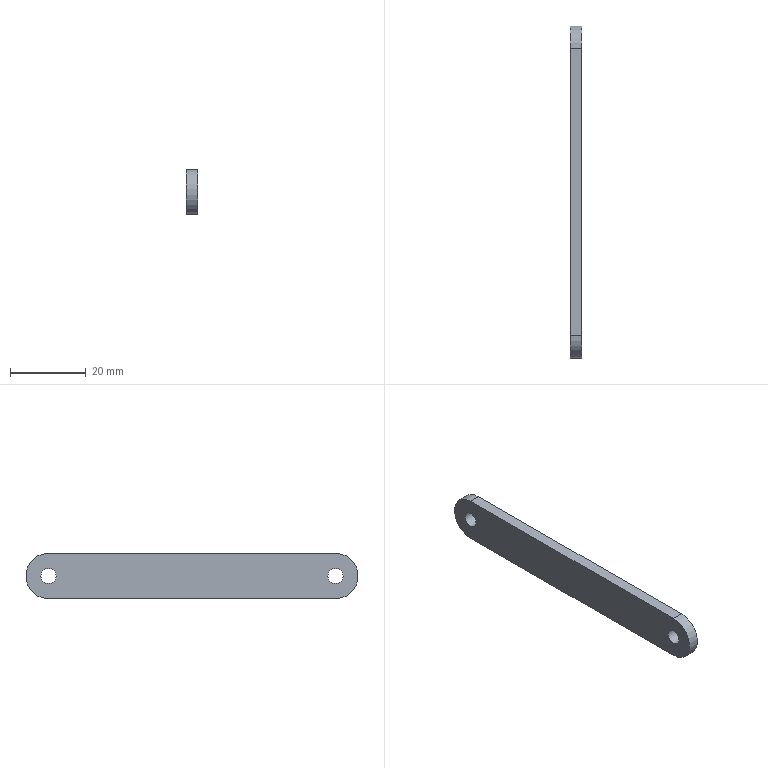Part | STEP file | 1-46.10 | 1 solid | 8 faces | box 3 x 88 x 12 mm | volume 3000 mm3 | plane 4 | cylinder 4 | commonest cylinder face diameters 4 x2 12 x2
STEP:
#1=CARTESIAN_POINT('',(0.,0.,0.));
#2=DIRECTION('',(0.,0.,1.));
#3=DIRECTION('',(1.,0.,0.));
#4=AXIS2_PLACEMENT_3D('',#1,#2,#3);
#5=CARTESIAN_POINT('',(0.,-38.,6.));
#6=VERTEX_POINT('',#5);
#7=CARTESIAN_POINT('',(0.,-38.,-6.));
#8=VERTEX_POINT('',#7);
#9=CARTESIAN_POINT('',(0.,-38.,0.));
#10=DIRECTION('',(1.,0.,0.));
#11=DIRECTION('',(0.,0.,1.));
#12=AXIS2_PLACEMENT_3D('',#9,#10,#11);
#13=CIRCLE('',#12,6.);
#14=CARTESIAN_POINT('',(0.,0.,38.));
#15=DIRECTION('',(1.,0.,0.));
#16=DIRECTION('',(0.,1.,0.));
#17=AXIS2_PLACEMENT_3D('',#14,#15,#16);
#18=PLANE('',#17);
#19=CARTESIAN_POINT('',(-38.,-38.));
#20=DIRECTION('',(0.,1.));
#21=AXIS2_PLACEMENT_2D('',#19,#20);
#22=CIRCLE('',#21,6.);
#23=(GEOMETRIC_REPRESENTATION_CONTEXT(2)PARAMETRIC_REPRESENTATION_CONTEXT()REPRESENTATION_CONTEXT('',''));
#24=DEFINITIONAL_REPRESENTATION('',(#22),#23);
#25=PCURVE('',#18,#24);
#26=CARTESIAN_POINT('',(0.,-38.,0.));
#27=DIRECTION('',(1.,0.,0.));
#28=DIRECTION('',(0.,0.,1.));
#29=AXIS2_PLACEMENT_3D('',#26,#27,#28);
#30=CYLINDRICAL_SURFACE('',#29,6.);
#31=CARTESIAN_POINT('',(0.,0.));
#32=DIRECTION('',(1.,0.));
#33=VECTOR('',#32,1.);
#34=LINE('',#31,#33);
#35=(GEOMETRIC_REPRESENTATION_CONTEXT(2)PARAMETRIC_REPRESENTATION_CONTEXT()REPRESENTATION_CONTEXT('',''));
#36=DEFINITIONAL_REPRESENTATION('',(#34),#35);
#37=PCURVE('',#30,#36);
#38=SURFACE_CURVE('',#13,(#25,#37),.PCURVE_S1.);
#39=EDGE_CURVE('',#6,#8,#38,.T.);
#40=ORIENTED_EDGE('',*,*,#39,.T.);
#41=CARTESIAN_POINT('',(0.,38.,-6.));
#42=VERTEX_POINT('',#41);
#43=CARTESIAN_POINT('',(0.,-38.,-6.));
#44=DIRECTION('',(0.,1.,0.));
#45=VECTOR('',#44,1.);
#46=LINE('',#43,#45);
#47=CARTESIAN_POINT('',(-38.,-44.));
#48=DIRECTION('',(1.,0.));
#49=VECTOR('',#48,1.);
#50=LINE('',#47,#49);
#51=(GEOMETRIC_REPRESENTATION_CONTEXT(2)PARAMETRIC_REPRESENTATION_CONTEXT()REPRESENTATION_CONTEXT('',''));
#52=DEFINITIONAL_REPRESENTATION('',(#50),#51);
#53=PCURVE('',#18,#52);
#54=CARTESIAN_POINT('',(1.5,0.,-6.));
#55=DIRECTION('',(0.,0.,-1.));
#56=DIRECTION('',(0.,1.,0.));
#57=AXIS2_PLACEMENT_3D('',#54,#55,#56);
#58=PLANE('',#57);
#59=CARTESIAN_POINT('',(-38.,-1.5));
#60=DIRECTION('',(1.,0.));
#61=VECTOR('',#60,1.);
#62=LINE('',#59,#61);
#63=(GEOMETRIC_REPRESENTATION_CONTEXT(2)PARAMETRIC_REPRESENTATION_CONTEXT()REPRESENTATION_CONTEXT('',''));
#64=DEFINITIONAL_REPRESENTATION('',(#62),#63);
#65=PCURVE('',#58,#64);
#66=SURFACE_CURVE('',#46,(#53,#65),.PCURVE_S1.);
#67=EDGE_CURVE('',#8,#42,#66,.T.);
#68=ORIENTED_EDGE('',*,*,#67,.T.);
#69=CARTESIAN_POINT('',(0.,38.,6.));
#70=VERTEX_POINT('',#69);
#71=CARTESIAN_POINT('',(0.,38.,0.));
#72=DIRECTION('',(1.,0.,0.));
#73=DIRECTION('',(0.,0.,-1.));
#74=AXIS2_PLACEMENT_3D('',#71,#72,#73);
#75=CIRCLE('',#74,6.);
#76=CARTESIAN_POINT('',(38.,-38.));
#77=DIRECTION('',(0.,-1.));
#78=AXIS2_PLACEMENT_2D('',#76,#77);
#79=CIRCLE('',#78,6.);
#80=(GEOMETRIC_REPRESENTATION_CONTEXT(2)PARAMETRIC_REPRESENTATION_CONTEXT()REPRESENTATION_CONTEXT('',''));
#81=DEFINITIONAL_REPRESENTATION('',(#79),#80);
#82=PCURVE('',#18,#81);
#83=CARTESIAN_POINT('',(0.,38.,0.));
#84=DIRECTION('',(1.,0.,0.));
#85=DIRECTION('',(0.,0.,-1.));
#86=AXIS2_PLACEMENT_3D('',#83,#84,#85);
#87=CYLINDRICAL_SURFACE('',#86,6.);
#88=CARTESIAN_POINT('',(0.,0.));
#89=DIRECTION('',(1.,0.));
#90=VECTOR('',#89,1.);
#91=LINE('',#88,#90);
#92=(GEOMETRIC_REPRESENTATION_CONTEXT(2)PARAMETRIC_REPRESENTATION_CONTEXT()REPRESENTATION_CONTEXT('',''));
#93=DEFINITIONAL_REPRESENTATION('',(#91),#92);
#94=PCURVE('',#87,#93);
#95=SURFACE_CURVE('',#75,(#82,#94),.PCURVE_S1.);
#96=EDGE_CURVE('',#42,#70,#95,.T.);
#97=ORIENTED_EDGE('',*,*,#96,.T.);
#98=CARTESIAN_POINT('',(0.,38.,6.));
#99=DIRECTION('',(0.,-1.,0.));
#100=VECTOR('',#99,1.);
#101=LINE('',#98,#100);
#102=CARTESIAN_POINT('',(38.,-32.));
#103=DIRECTION('',(-1.,0.));
#104=VECTOR('',#103,1.);
#105=LINE('',#102,#104);
#106=(GEOMETRIC_REPRESENTATION_CONTEXT(2)PARAMETRIC_REPRESENTATION_CONTEXT()REPRESENTATION_CONTEXT('',''));
#107=DEFINITIONAL_REPRESENTATION('',(#105),#106);
#108=PCURVE('',#18,#107);
#109=CARTESIAN_POINT('',(1.5,0.,6.));
#110=DIRECTION('',(0.,0.,1.));
#111=DIRECTION('',(0.,-1.,0.));
#112=AXIS2_PLACEMENT_3D('',#109,#110,#111);
#113=PLANE('',#112);
#114=CARTESIAN_POINT('',(-38.,-1.5));
#115=DIRECTION('',(1.,0.));
#116=VECTOR('',#115,1.);
#117=LINE('',#114,#116);
#118=(GEOMETRIC_REPRESENTATION_CONTEXT(2)PARAMETRIC_REPRESENTATION_CONTEXT()REPRESENTATION_CONTEXT('',''));
#119=DEFINITIONAL_REPRESENTATION('',(#117),#118);
#120=PCURVE('',#113,#119);
#121=SURFACE_CURVE('',#101,(#108,#120),.PCURVE_S1.);
#122=EDGE_CURVE('',#70,#6,#121,.T.);
#123=ORIENTED_EDGE('',*,*,#122,.T.);
#124=EDGE_LOOP('',(#40,#68,#97,#123));
#125=FACE_BOUND('',#124,.F.);
#126=CARTESIAN_POINT('',(0.,-36.,0.));
#127=VERTEX_POINT('',#126);
#128=CARTESIAN_POINT('',(0.,-38.,0.));
#129=DIRECTION('',(-1.,0.,0.));
#130=DIRECTION('',(0.,1.,0.));
#131=AXIS2_PLACEMENT_3D('',#128,#129,#130);
#132=CIRCLE('',#131,2.);
#133=CARTESIAN_POINT('',(-36.,-38.));
#134=CARTESIAN_POINT('',(-36.,-41.464));
#135=CARTESIAN_POINT('',(-39.,-39.732));
#136=CARTESIAN_POINT('',(-42.,-38.));
#137=CARTESIAN_POINT('',(-39.,-36.268));
#138=CARTESIAN_POINT('',(-36.,-34.536));
#139=CARTESIAN_POINT('',(-36.,-38.));
#140=(BOUNDED_CURVE()B_SPLINE_CURVE(2,(#133,#134,#135,#136,#137,#138,#139),.UNSPECIFIED.,.T.,.F.)B_SPLINE_CURVE_WITH_KNOTS((1,2,2,2,2,1),(-2.094,0.,2.094,4.189,6.283,8.378),.UNSPECIFIED.)CURVE()GEOMETRIC_REPRESENTATION_ITEM()RATIONAL_B_SPLINE_CURVE((1.,0.5,1.,0.5,1.,0.5,1.))REPRESENTATION_ITEM(''));
#141=(GEOMETRIC_REPRESENTATION_CONTEXT(2)PARAMETRIC_REPRESENTATION_CONTEXT()REPRESENTATION_CONTEXT('',''));
#142=DEFINITIONAL_REPRESENTATION('',(#140),#141);
#143=PCURVE('',#18,#142);
#144=CARTESIAN_POINT('',(0.,-38.,0.));
#145=DIRECTION('',(1.,0.,0.));
#146=DIRECTION('',(0.,1.,0.));
#147=AXIS2_PLACEMENT_3D('',#144,#145,#146);
#148=CYLINDRICAL_SURFACE('',#147,2.);
#149=CARTESIAN_POINT('',(6.283,0.));
#150=DIRECTION('',(-1.,0.));
#151=VECTOR('',#150,1.);
#152=LINE('',#149,#151);
#153=(GEOMETRIC_REPRESENTATION_CONTEXT(2)PARAMETRIC_REPRESENTATION_CONTEXT()REPRESENTATION_CONTEXT('',''));
#154=DEFINITIONAL_REPRESENTATION('',(#152),#153);
#155=PCURVE('',#148,#154);
#156=SURFACE_CURVE('',#132,(#143,#155),.PCURVE_S1.);
#157=EDGE_CURVE('',#127,#127,#156,.T.);
#158=ORIENTED_EDGE('',*,*,#157,.T.);
#159=EDGE_LOOP('',(#158));
#160=FACE_BOUND('',#159,.F.);
#161=CARTESIAN_POINT('',(0.,40.,0.));
#162=VERTEX_POINT('',#161);
#163=CARTESIAN_POINT('',(0.,38.,0.));
#164=DIRECTION('',(-1.,0.,0.));
#165=DIRECTION('',(0.,1.,0.));
#166=AXIS2_PLACEMENT_3D('',#163,#164,#165);
#167=CIRCLE('',#166,2.);
#168=CARTESIAN_POINT('',(40.,-38.));
#169=CARTESIAN_POINT('',(40.,-41.464));
#170=CARTESIAN_POINT('',(37.,-39.732));
#171=CARTESIAN_POINT('',(34.,-38.));
#172=CARTESIAN_POINT('',(37.,-36.268));
#173=CARTESIAN_POINT('',(40.,-34.536));
#174=CARTESIAN_POINT('',(40.,-38.));
#175=(BOUNDED_CURVE()B_SPLINE_CURVE(2,(#168,#169,#170,#171,#172,#173,#174),.UNSPECIFIED.,.T.,.F.)B_SPLINE_CURVE_WITH_KNOTS((1,2,2,2,2,1),(-2.094,0.,2.094,4.189,6.283,8.378),.UNSPECIFIED.)CURVE()GEOMETRIC_REPRESENTATION_ITEM()RATIONAL_B_SPLINE_CURVE((1.,0.5,1.,0.5,1.,0.5,1.))REPRESENTATION_ITEM(''));
#176=(GEOMETRIC_REPRESENTATION_CONTEXT(2)PARAMETRIC_REPRESENTATION_CONTEXT()REPRESENTATION_CONTEXT('',''));
#177=DEFINITIONAL_REPRESENTATION('',(#175),#176);
#178=PCURVE('',#18,#177);
#179=CARTESIAN_POINT('',(0.,38.,0.));
#180=DIRECTION('',(1.,0.,0.));
#181=DIRECTION('',(0.,1.,0.));
#182=AXIS2_PLACEMENT_3D('',#179,#180,#181);
#183=CYLINDRICAL_SURFACE('',#182,2.);
#184=CARTESIAN_POINT('',(6.283,0.));
#185=DIRECTION('',(-1.,0.));
#186=VECTOR('',#185,1.);
#187=LINE('',#184,#186);
#188=(GEOMETRIC_REPRESENTATION_CONTEXT(2)PARAMETRIC_REPRESENTATION_CONTEXT()REPRESENTATION_CONTEXT('',''));
#189=DEFINITIONAL_REPRESENTATION('',(#187),#188);
#190=PCURVE('',#183,#189);
#191=SURFACE_CURVE('',#167,(#178,#190),.PCURVE_S1.);
#192=EDGE_CURVE('',#162,#162,#191,.T.);
#193=ORIENTED_EDGE('',*,*,#192,.T.);
#194=EDGE_LOOP('',(#193));
#195=FACE_BOUND('',#194,.F.);
#196=ADVANCED_FACE('',(#125,#160,#195),#18,.F.);
#197=CARTESIAN_POINT('',(3.,-38.,6.));
#198=VERTEX_POINT('',#197);
#199=CARTESIAN_POINT('',(3.,-38.,-6.));
#200=VERTEX_POINT('',#199);
#201=CARTESIAN_POINT('',(3.,-38.,0.));
#202=DIRECTION('',(1.,0.,0.));
#203=DIRECTION('',(0.,0.,1.));
#204=AXIS2_PLACEMENT_3D('',#201,#202,#203);
#205=CIRCLE('',#204,6.);
#206=CARTESIAN_POINT('',(3.,0.,38.));
#207=DIRECTION('',(1.,0.,0.));
#208=DIRECTION('',(0.,1.,0.));
#209=AXIS2_PLACEMENT_3D('',#206,#207,#208);
#210=PLANE('',#209);
#211=CARTESIAN_POINT('',(-38.,-38.));
#212=DIRECTION('',(0.,1.));
#213=AXIS2_PLACEMENT_2D('',#211,#212);
#214=CIRCLE('',#213,6.);
#215=(GEOMETRIC_REPRESENTATION_CONTEXT(2)PARAMETRIC_REPRESENTATION_CONTEXT()REPRESENTATION_CONTEXT('',''));
#216=DEFINITIONAL_REPRESENTATION('',(#214),#215);
#217=PCURVE('',#210,#216);
#218=CARTESIAN_POINT('',(0.,3.));
#219=DIRECTION('',(1.,0.));
#220=VECTOR('',#219,1.);
#221=LINE('',#218,#220);
#222=(GEOMETRIC_REPRESENTATION_CONTEXT(2)PARAMETRIC_REPRESENTATION_CONTEXT()REPRESENTATION_CONTEXT('',''));
#223=DEFINITIONAL_REPRESENTATION('',(#221),#222);
#224=PCURVE('',#30,#223);
#225=SURFACE_CURVE('',#205,(#217,#224),.PCURVE_S1.);
#226=EDGE_CURVE('',#198,#200,#225,.T.);
#227=ORIENTED_EDGE('',*,*,#226,.T.);
#228=CARTESIAN_POINT('',(3.,38.,-6.));
#229=VERTEX_POINT('',#228);
#230=CARTESIAN_POINT('',(3.,-38.,-6.));
#231=DIRECTION('',(0.,1.,0.));
#232=VECTOR('',#231,1.);
#233=LINE('',#230,#232);
#234=CARTESIAN_POINT('',(-38.,-44.));
#235=DIRECTION('',(1.,0.));
#236=VECTOR('',#235,1.);
#237=LINE('',#234,#236);
#238=(GEOMETRIC_REPRESENTATION_CONTEXT(2)PARAMETRIC_REPRESENTATION_CONTEXT()REPRESENTATION_CONTEXT('',''));
#239=DEFINITIONAL_REPRESENTATION('',(#237),#238);
#240=PCURVE('',#210,#239);
#241=CARTESIAN_POINT('',(-38.,1.5));
#242=DIRECTION('',(1.,0.));
#243=VECTOR('',#242,1.);
#244=LINE('',#241,#243);
#245=(GEOMETRIC_REPRESENTATION_CONTEXT(2)PARAMETRIC_REPRESENTATION_CONTEXT()REPRESENTATION_CONTEXT('',''));
#246=DEFINITIONAL_REPRESENTATION('',(#244),#245);
#247=PCURVE('',#58,#246);
#248=SURFACE_CURVE('',#233,(#240,#247),.PCURVE_S1.);
#249=EDGE_CURVE('',#200,#229,#248,.T.);
#250=ORIENTED_EDGE('',*,*,#249,.T.);
#251=CARTESIAN_POINT('',(3.,38.,6.));
#252=VERTEX_POINT('',#251);
#253=CARTESIAN_POINT('',(3.,38.,0.));
#254=DIRECTION('',(1.,0.,0.));
#255=DIRECTION('',(0.,0.,-1.));
#256=AXIS2_PLACEMENT_3D('',#253,#254,#255);
#257=CIRCLE('',#256,6.);
#258=CARTESIAN_POINT('',(38.,-38.));
#259=DIRECTION('',(0.,-1.));
#260=AXIS2_PLACEMENT_2D('',#258,#259);
#261=CIRCLE('',#260,6.);
#262=(GEOMETRIC_REPRESENTATION_CONTEXT(2)PARAMETRIC_REPRESENTATION_CONTEXT()REPRESENTATION_CONTEXT('',''));
#263=DEFINITIONAL_REPRESENTATION('',(#261),#262);
#264=PCURVE('',#210,#263);
#265=CARTESIAN_POINT('',(0.,3.));
#266=DIRECTION('',(1.,0.));
#267=VECTOR('',#266,1.);
#268=LINE('',#265,#267);
#269=(GEOMETRIC_REPRESENTATION_CONTEXT(2)PARAMETRIC_REPRESENTATION_CONTEXT()REPRESENTATION_CONTEXT('',''));
#270=DEFINITIONAL_REPRESENTATION('',(#268),#269);
#271=PCURVE('',#87,#270);
#272=SURFACE_CURVE('',#257,(#264,#271),.PCURVE_S1.);
#273=EDGE_CURVE('',#229,#252,#272,.T.);
#274=ORIENTED_EDGE('',*,*,#273,.T.);
#275=CARTESIAN_POINT('',(3.,38.,6.));
#276=DIRECTION('',(0.,-1.,0.));
#277=VECTOR('',#276,1.);
#278=LINE('',#275,#277);
#279=CARTESIAN_POINT('',(38.,-32.));
#280=DIRECTION('',(-1.,0.));
#281=VECTOR('',#280,1.);
#282=LINE('',#279,#281);
#283=(GEOMETRIC_REPRESENTATION_CONTEXT(2)PARAMETRIC_REPRESENTATION_CONTEXT()REPRESENTATION_CONTEXT('',''));
#284=DEFINITIONAL_REPRESENTATION('',(#282),#283);
#285=PCURVE('',#210,#284);
#286=CARTESIAN_POINT('',(-38.,1.5));
#287=DIRECTION('',(1.,0.));
#288=VECTOR('',#287,1.);
#289=LINE('',#286,#288);
#290=(GEOMETRIC_REPRESENTATION_CONTEXT(2)PARAMETRIC_REPRESENTATION_CONTEXT()REPRESENTATION_CONTEXT('',''));
#291=DEFINITIONAL_REPRESENTATION('',(#289),#290);
#292=PCURVE('',#113,#291);
#293=SURFACE_CURVE('',#278,(#285,#292),.PCURVE_S1.);
#294=EDGE_CURVE('',#252,#198,#293,.T.);
#295=ORIENTED_EDGE('',*,*,#294,.T.);
#296=EDGE_LOOP('',(#227,#250,#274,#295));
#297=FACE_BOUND('',#296,.T.);
#298=CARTESIAN_POINT('',(3.,-36.,0.));
#299=VERTEX_POINT('',#298);
#300=CARTESIAN_POINT('',(3.,-38.,0.));
#301=DIRECTION('',(-1.,0.,0.));
#302=DIRECTION('',(0.,1.,0.));
#303=AXIS2_PLACEMENT_3D('',#300,#301,#302);
#304=CIRCLE('',#303,2.);
#305=CARTESIAN_POINT('',(-36.,-38.));
#306=CARTESIAN_POINT('',(-36.,-41.464));
#307=CARTESIAN_POINT('',(-39.,-39.732));
#308=CARTESIAN_POINT('',(-42.,-38.));
#309=CARTESIAN_POINT('',(-39.,-36.268));
#310=CARTESIAN_POINT('',(-36.,-34.536));
#311=CARTESIAN_POINT('',(-36.,-38.));
#312=(BOUNDED_CURVE()B_SPLINE_CURVE(2,(#305,#306,#307,#308,#309,#310,#311),.UNSPECIFIED.,.T.,.F.)B_SPLINE_CURVE_WITH_KNOTS((1,2,2,2,2,1),(-2.094,0.,2.094,4.189,6.283,8.378),.UNSPECIFIED.)CURVE()GEOMETRIC_REPRESENTATION_ITEM()RATIONAL_B_SPLINE_CURVE((1.,0.5,1.,0.5,1.,0.5,1.))REPRESENTATION_ITEM(''));
#313=(GEOMETRIC_REPRESENTATION_CONTEXT(2)PARAMETRIC_REPRESENTATION_CONTEXT()REPRESENTATION_CONTEXT('',''));
#314=DEFINITIONAL_REPRESENTATION('',(#312),#313);
#315=PCURVE('',#210,#314);
#316=CARTESIAN_POINT('',(6.283,3.));
#317=DIRECTION('',(-1.,0.));
#318=VECTOR('',#317,1.);
#319=LINE('',#316,#318);
#320=(GEOMETRIC_REPRESENTATION_CONTEXT(2)PARAMETRIC_REPRESENTATION_CONTEXT()REPRESENTATION_CONTEXT('',''));
#321=DEFINITIONAL_REPRESENTATION('',(#319),#320);
#322=PCURVE('',#148,#321);
#323=SURFACE_CURVE('',#304,(#315,#322),.PCURVE_S1.);
#324=EDGE_CURVE('',#299,#299,#323,.T.);
#325=ORIENTED_EDGE('',*,*,#324,.T.);
#326=EDGE_LOOP('',(#325));
#327=FACE_BOUND('',#326,.T.);
#328=CARTESIAN_POINT('',(3.,40.,0.));
#329=VERTEX_POINT('',#328);
#330=CARTESIAN_POINT('',(3.,38.,0.));
#331=DIRECTION('',(-1.,0.,0.));
#332=DIRECTION('',(0.,1.,0.));
#333=AXIS2_PLACEMENT_3D('',#330,#331,#332);
#334=CIRCLE('',#333,2.);
#335=CARTESIAN_POINT('',(40.,-38.));
#336=CARTESIAN_POINT('',(40.,-41.464));
#337=CARTESIAN_POINT('',(37.,-39.732));
#338=CARTESIAN_POINT('',(34.,-38.));
#339=CARTESIAN_POINT('',(37.,-36.268));
#340=CARTESIAN_POINT('',(40.,-34.536));
#341=CARTESIAN_POINT('',(40.,-38.));
#342=(BOUNDED_CURVE()B_SPLINE_CURVE(2,(#335,#336,#337,#338,#339,#340,#341),.UNSPECIFIED.,.T.,.F.)B_SPLINE_CURVE_WITH_KNOTS((1,2,2,2,2,1),(-2.094,0.,2.094,4.189,6.283,8.378),.UNSPECIFIED.)CURVE()GEOMETRIC_REPRESENTATION_ITEM()RATIONAL_B_SPLINE_CURVE((1.,0.5,1.,0.5,1.,0.5,1.))REPRESENTATION_ITEM(''));
#343=(GEOMETRIC_REPRESENTATION_CONTEXT(2)PARAMETRIC_REPRESENTATION_CONTEXT()REPRESENTATION_CONTEXT('',''));
#344=DEFINITIONAL_REPRESENTATION('',(#342),#343);
#345=PCURVE('',#210,#344);
#346=CARTESIAN_POINT('',(6.283,3.));
#347=DIRECTION('',(-1.,0.));
#348=VECTOR('',#347,1.);
#349=LINE('',#346,#348);
#350=(GEOMETRIC_REPRESENTATION_CONTEXT(2)PARAMETRIC_REPRESENTATION_CONTEXT()REPRESENTATION_CONTEXT('',''));
#351=DEFINITIONAL_REPRESENTATION('',(#349),#350);
#352=PCURVE('',#183,#351);
#353=SURFACE_CURVE('',#334,(#345,#352),.PCURVE_S1.);
#354=EDGE_CURVE('',#329,#329,#353,.T.);
#355=ORIENTED_EDGE('',*,*,#354,.T.);
#356=EDGE_LOOP('',(#355));
#357=FACE_BOUND('',#356,.T.);
#358=ADVANCED_FACE('',(#297,#327,#357),#210,.T.);
#359=ORIENTED_EDGE('',*,*,#39,.T.);
#360=CARTESIAN_POINT('',(0.,-38.,-6.));
#361=DIRECTION('',(1.,0.,0.));
#362=VECTOR('',#361,1.);
#363=LINE('',#360,#362);
#364=CARTESIAN_POINT('',(3.142,0.));
#365=DIRECTION('',(0.,1.));
#366=VECTOR('',#365,1.);
#367=LINE('',#364,#366);
#368=(GEOMETRIC_REPRESENTATION_CONTEXT(2)PARAMETRIC_REPRESENTATION_CONTEXT()REPRESENTATION_CONTEXT('',''));
#369=DEFINITIONAL_REPRESENTATION('',(#367),#368);
#370=PCURVE('',#30,#369);
#371=CARTESIAN_POINT('',(-38.,-1.5));
#372=DIRECTION('',(0.,1.));
#373=VECTOR('',#372,1.);
#374=LINE('',#371,#373);
#375=(GEOMETRIC_REPRESENTATION_CONTEXT(2)PARAMETRIC_REPRESENTATION_CONTEXT()REPRESENTATION_CONTEXT('',''));
#376=DEFINITIONAL_REPRESENTATION('',(#374),#375);
#377=PCURVE('',#58,#376);
#378=SURFACE_CURVE('',#363,(#370,#377),.PCURVE_S1.);
#379=EDGE_CURVE('',#8,#200,#378,.T.);
#380=ORIENTED_EDGE('',*,*,#379,.T.);
#381=ORIENTED_EDGE('',*,*,#226,.F.);
#382=CARTESIAN_POINT('',(0.,-38.,6.));
#383=DIRECTION('',(1.,0.,0.));
#384=VECTOR('',#383,1.);
#385=LINE('',#382,#384);
#386=CARTESIAN_POINT('',(0.,0.));
#387=DIRECTION('',(0.,1.));
#388=VECTOR('',#387,1.);
#389=LINE('',#386,#388);
#390=(GEOMETRIC_REPRESENTATION_CONTEXT(2)PARAMETRIC_REPRESENTATION_CONTEXT()REPRESENTATION_CONTEXT('',''));
#391=DEFINITIONAL_REPRESENTATION('',(#389),#390);
#392=PCURVE('',#30,#391);
#393=CARTESIAN_POINT('',(38.,-1.5));
#394=DIRECTION('',(0.,1.));
#395=VECTOR('',#394,1.);
#396=LINE('',#393,#395);
#397=(GEOMETRIC_REPRESENTATION_CONTEXT(2)PARAMETRIC_REPRESENTATION_CONTEXT()REPRESENTATION_CONTEXT('',''));
#398=DEFINITIONAL_REPRESENTATION('',(#396),#397);
#399=PCURVE('',#113,#398);
#400=SURFACE_CURVE('',#385,(#392,#399),.PCURVE_S1.);
#401=EDGE_CURVE('',#6,#198,#400,.T.);
#402=ORIENTED_EDGE('',*,*,#401,.F.);
#403=EDGE_LOOP('',(#359,#380,#381,#402));
#404=FACE_BOUND('',#403,.T.);
#405=ADVANCED_FACE('',(#404),#30,.T.);
#406=ORIENTED_EDGE('',*,*,#67,.T.);
#407=CARTESIAN_POINT('',(0.,38.,-6.));
#408=DIRECTION('',(1.,0.,0.));
#409=VECTOR('',#408,1.);
#410=LINE('',#407,#409);
#411=CARTESIAN_POINT('',(38.,-1.5));
#412=DIRECTION('',(0.,1.));
#413=VECTOR('',#412,1.);
#414=LINE('',#411,#413);
#415=(GEOMETRIC_REPRESENTATION_CONTEXT(2)PARAMETRIC_REPRESENTATION_CONTEXT()REPRESENTATION_CONTEXT('',''));
#416=DEFINITIONAL_REPRESENTATION('',(#414),#415);
#417=PCURVE('',#58,#416);
#418=CARTESIAN_POINT('',(0.,0.));
#419=DIRECTION('',(0.,1.));
#420=VECTOR('',#419,1.);
#421=LINE('',#418,#420);
#422=(GEOMETRIC_REPRESENTATION_CONTEXT(2)PARAMETRIC_REPRESENTATION_CONTEXT()REPRESENTATION_CONTEXT('',''));
#423=DEFINITIONAL_REPRESENTATION('',(#421),#422);
#424=PCURVE('',#87,#423);
#425=SURFACE_CURVE('',#410,(#417,#424),.PCURVE_S1.);
#426=EDGE_CURVE('',#42,#229,#425,.T.);
#427=ORIENTED_EDGE('',*,*,#426,.T.);
#428=ORIENTED_EDGE('',*,*,#249,.F.);
#429=ORIENTED_EDGE('',*,*,#379,.F.);
#430=EDGE_LOOP('',(#406,#427,#428,#429));
#431=FACE_BOUND('',#430,.T.);
#432=ADVANCED_FACE('',(#431),#58,.T.);
#433=ORIENTED_EDGE('',*,*,#96,.T.);
#434=CARTESIAN_POINT('',(0.,38.,6.));
#435=DIRECTION('',(1.,0.,0.));
#436=VECTOR('',#435,1.);
#437=LINE('',#434,#436);
#438=CARTESIAN_POINT('',(3.142,0.));
#439=DIRECTION('',(0.,1.));
#440=VECTOR('',#439,1.);
#441=LINE('',#438,#440);
#442=(GEOMETRIC_REPRESENTATION_CONTEXT(2)PARAMETRIC_REPRESENTATION_CONTEXT()REPRESENTATION_CONTEXT('',''));
#443=DEFINITIONAL_REPRESENTATION('',(#441),#442);
#444=PCURVE('',#87,#443);
#445=CARTESIAN_POINT('',(-38.,-1.5));
#446=DIRECTION('',(0.,1.));
#447=VECTOR('',#446,1.);
#448=LINE('',#445,#447);
#449=(GEOMETRIC_REPRESENTATION_CONTEXT(2)PARAMETRIC_REPRESENTATION_CONTEXT()REPRESENTATION_CONTEXT('',''));
#450=DEFINITIONAL_REPRESENTATION('',(#448),#449);
#451=PCURVE('',#113,#450);
#452=SURFACE_CURVE('',#437,(#444,#451),.PCURVE_S1.);
#453=EDGE_CURVE('',#70,#252,#452,.T.);
#454=ORIENTED_EDGE('',*,*,#453,.T.);
#455=ORIENTED_EDGE('',*,*,#273,.F.);
#456=ORIENTED_EDGE('',*,*,#426,.F.);
#457=EDGE_LOOP('',(#433,#454,#455,#456));
#458=FACE_BOUND('',#457,.T.);
#459=ADVANCED_FACE('',(#458),#87,.T.);
#460=ORIENTED_EDGE('',*,*,#122,.T.);
#461=ORIENTED_EDGE('',*,*,#401,.T.);
#462=ORIENTED_EDGE('',*,*,#294,.F.);
#463=ORIENTED_EDGE('',*,*,#453,.F.);
#464=EDGE_LOOP('',(#460,#461,#462,#463));
#465=FACE_BOUND('',#464,.T.);
#466=ADVANCED_FACE('',(#465),#113,.T.);
#467=CARTESIAN_POINT('',(0.,-36.,0.));
#468=DIRECTION('',(1.,0.,0.));
#469=VECTOR('',#468,1.);
#470=LINE('',#467,#469);
#471=CARTESIAN_POINT('',(6.283,0.));
#472=DIRECTION('',(0.,1.));
#473=VECTOR('',#472,1.);
#474=LINE('',#471,#473);
#475=(GEOMETRIC_REPRESENTATION_CONTEXT(2)PARAMETRIC_REPRESENTATION_CONTEXT()REPRESENTATION_CONTEXT('',''));
#476=DEFINITIONAL_REPRESENTATION('',(#474),#475);
#477=PCURVE('',#148,#476);
#478=CARTESIAN_POINT('',(0.,0.));
#479=DIRECTION('',(0.,1.));
#480=VECTOR('',#479,1.);
#481=LINE('',#478,#480);
#482=(GEOMETRIC_REPRESENTATION_CONTEXT(2)PARAMETRIC_REPRESENTATION_CONTEXT()REPRESENTATION_CONTEXT('',''));
#483=DEFINITIONAL_REPRESENTATION('',(#481),#482);
#484=PCURVE('',#148,#483);
#485=SEAM_CURVE('',#470,(#477,#484),.PCURVE_S1.);
#486=EDGE_CURVE('',#127,#299,#485,.T.);
#487=ORIENTED_EDGE('',*,*,#486,.T.);
#488=ORIENTED_EDGE('',*,*,#324,.T.);
#489=ORIENTED_EDGE('',*,*,#486,.F.);
#490=ORIENTED_EDGE('',*,*,#157,.F.);
#491=EDGE_LOOP('',(#487,#488,#489,#490));
#492=FACE_BOUND('',#491,.F.);
#493=ADVANCED_FACE('',(#492),#148,.F.);
#494=CARTESIAN_POINT('',(0.,40.,0.));
#495=DIRECTION('',(1.,0.,0.));
#496=VECTOR('',#495,1.);
#497=LINE('',#494,#496);
#498=CARTESIAN_POINT('',(6.283,0.));
#499=DIRECTION('',(0.,1.));
#500=VECTOR('',#499,1.);
#501=LINE('',#498,#500);
#502=(GEOMETRIC_REPRESENTATION_CONTEXT(2)PARAMETRIC_REPRESENTATION_CONTEXT()REPRESENTATION_CONTEXT('',''));
#503=DEFINITIONAL_REPRESENTATION('',(#501),#502);
#504=PCURVE('',#183,#503);
#505=CARTESIAN_POINT('',(0.,0.));
#506=DIRECTION('',(0.,1.));
#507=VECTOR('',#506,1.);
#508=LINE('',#505,#507);
#509=(GEOMETRIC_REPRESENTATION_CONTEXT(2)PARAMETRIC_REPRESENTATION_CONTEXT()REPRESENTATION_CONTEXT('',''));
#510=DEFINITIONAL_REPRESENTATION('',(#508),#509);
#511=PCURVE('',#183,#510);
#512=SEAM_CURVE('',#497,(#504,#511),.PCURVE_S1.);
#513=EDGE_CURVE('',#162,#329,#512,.T.);
#514=ORIENTED_EDGE('',*,*,#513,.T.);
#515=ORIENTED_EDGE('',*,*,#354,.T.);
#516=ORIENTED_EDGE('',*,*,#513,.F.);
#517=ORIENTED_EDGE('',*,*,#192,.F.);
#518=EDGE_LOOP('',(#514,#515,#516,#517));
#519=FACE_BOUND('',#518,.F.);
#520=ADVANCED_FACE('',(#519),#183,.F.);
#521=CLOSED_SHELL('',(#196,#358,#405,#432,#459,#466,#493,#520));
#522=MANIFOLD_SOLID_BREP('',#521);
#523=(LENGTH_UNIT()NAMED_UNIT(*)SI_UNIT(.MILLI.,.METRE.));
#524=UNCERTAINTY_MEASURE_WITH_UNIT(LENGTH_MEASURE(0.0000001),#523,'','');
#525=(NAMED_UNIT(*)PLANE_ANGLE_UNIT()SI_UNIT($,.RADIAN.));
#526=(NAMED_UNIT(*)SI_UNIT($,.STERADIAN.)SOLID_ANGLE_UNIT());
#527=(GEOMETRIC_REPRESENTATION_CONTEXT(3)GLOBAL_UNCERTAINTY_ASSIGNED_CONTEXT((#524))GLOBAL_UNIT_ASSIGNED_CONTEXT((#523,#525,#526))REPRESENTATION_CONTEXT('',''));
#528=ADVANCED_BREP_SHAPE_REPRESENTATION('',(#4,#522),#527);